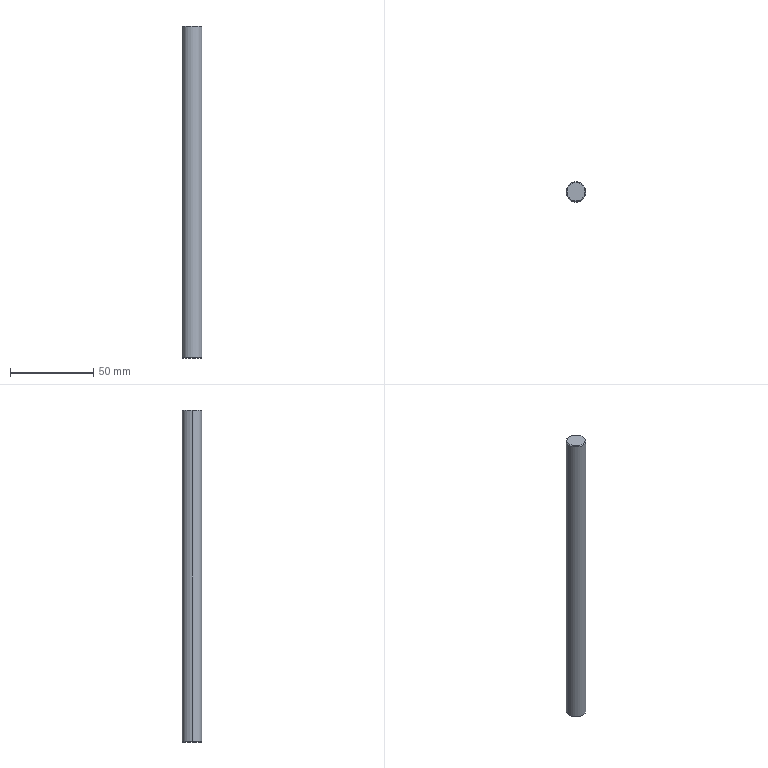Part | SolidWorks | features Chamfer 1, Extrusion 1 | 1 solid | 8 faces | box 12 x 12 x 200 mm | volume 22610 mm3 | cone 4 | cylinder 2 | plane 2 | commonest cylinder face diameters 12 x2
STEP:
#1=CARTESIAN_POINT('',(5.5,0.,100.));
#2=VERTEX_POINT('',#1);
#3=CARTESIAN_POINT('',(-5.5,0.,100.));
#4=VERTEX_POINT('',#3);
#5=CARTESIAN_POINT('',(0.,0.,100.));
#6=DIRECTION('',(0.,0.,1.));
#7=DIRECTION('',(1.,0.,0.));
#8=AXIS2_PLACEMENT_3D('',#5,#6,#7);
#9=CIRCLE('',#8,5.5);
#10=EDGE_CURVE('',#2,#4,#9,.T.);
#11=ORIENTED_EDGE('',*,*,#10,.F.);
#12=CARTESIAN_POINT('',(6.,0.,99.5));
#13=VERTEX_POINT('',#12);
#14=CARTESIAN_POINT('',(5.5,0.,100.));
#15=DIRECTION('',(0.7071,0.,-0.7071));
#16=VECTOR('',#15,1000.);
#17=LINE('',#14,#16);
#18=EDGE_CURVE('',#2,#13,#17,.T.);
#19=ORIENTED_EDGE('',*,*,#18,.T.);
#20=CARTESIAN_POINT('',(-6.,0.,99.5));
#21=VERTEX_POINT('',#20);
#22=CARTESIAN_POINT('',(0.,0.,99.5));
#23=DIRECTION('',(0.,0.,-1.));
#24=DIRECTION('',(1.,0.,0.));
#25=AXIS2_PLACEMENT_3D('',#22,#23,#24);
#26=CIRCLE('',#25,6.);
#27=EDGE_CURVE('',#21,#13,#26,.T.);
#28=ORIENTED_EDGE('',*,*,#27,.F.);
#29=CARTESIAN_POINT('',(-5.5,0.,100.));
#30=DIRECTION('',(-0.7071,0.,-0.7071));
#31=VECTOR('',#30,1000.);
#32=LINE('',#29,#31);
#33=EDGE_CURVE('',#4,#21,#32,.T.);
#34=ORIENTED_EDGE('',*,*,#33,.F.);
#35=EDGE_LOOP('',(#11,#19,#28,#34));
#36=FACE_OUTER_BOUND('',#35,.T.);
#37=CARTESIAN_POINT('',(0.,0.,100.));
#38=DIRECTION('',(0.,0.,-1.));
#39=DIRECTION('',(-1.,0.,0.));
#40=AXIS2_PLACEMENT_3D('',#37,#38,#39);
#41=CONICAL_SURFACE('',#40,5.5,0.7854);
#42=ADVANCED_FACE('',(#36),#41,.T.);
#43=CARTESIAN_POINT('',(-5.5,0.,-100.));
#44=VERTEX_POINT('',#43);
#45=CARTESIAN_POINT('',(5.5,0.,-100.));
#46=VERTEX_POINT('',#45);
#47=CARTESIAN_POINT('',(0.,0.,-100.));
#48=DIRECTION('',(0.,0.,-1.));
#49=DIRECTION('',(1.,0.,0.));
#50=AXIS2_PLACEMENT_3D('',#47,#48,#49);
#51=CIRCLE('',#50,5.5);
#52=EDGE_CURVE('',#44,#46,#51,.T.);
#53=ORIENTED_EDGE('',*,*,#52,.F.);
#54=CARTESIAN_POINT('',(-6.,0.,-99.5));
#55=VERTEX_POINT('',#54);
#56=CARTESIAN_POINT('',(-6.,0.,-99.5));
#57=DIRECTION('',(-0.7071,0.,0.7071));
#58=VECTOR('',#57,1000.);
#59=LINE('',#56,#58);
#60=EDGE_CURVE('',#44,#55,#59,.T.);
#61=ORIENTED_EDGE('',*,*,#60,.T.);
#62=CARTESIAN_POINT('',(6.,0.,-99.5));
#63=VERTEX_POINT('',#62);
#64=CARTESIAN_POINT('',(0.,0.,-99.5));
#65=DIRECTION('',(0.,0.,1.));
#66=DIRECTION('',(1.,0.,0.));
#67=AXIS2_PLACEMENT_3D('',#64,#65,#66);
#68=CIRCLE('',#67,6.);
#69=EDGE_CURVE('',#63,#55,#68,.T.);
#70=ORIENTED_EDGE('',*,*,#69,.F.);
#71=CARTESIAN_POINT('',(6.,0.,-99.5));
#72=DIRECTION('',(0.7071,0.,0.7071));
#73=VECTOR('',#72,1000.);
#74=LINE('',#71,#73);
#75=EDGE_CURVE('',#46,#63,#74,.T.);
#76=ORIENTED_EDGE('',*,*,#75,.F.);
#77=EDGE_LOOP('',(#53,#61,#70,#76));
#78=FACE_OUTER_BOUND('',#77,.T.);
#79=CARTESIAN_POINT('',(0.,0.,-99.5));
#80=DIRECTION('',(0.,0.,1.));
#81=DIRECTION('',(1.,0.,0.));
#82=AXIS2_PLACEMENT_3D('',#79,#80,#81);
#83=CONICAL_SURFACE('',#82,6.,0.7854);
#84=ADVANCED_FACE('',(#78),#83,.T.);
#85=ORIENTED_EDGE('',*,*,#27,.T.);
#86=CARTESIAN_POINT('',(6.,0.,100.));
#87=DIRECTION('',(0.,0.,-1.));
#88=VECTOR('',#87,1000.);
#89=LINE('',#86,#88);
#90=EDGE_CURVE('',#13,#63,#89,.T.);
#91=ORIENTED_EDGE('',*,*,#90,.T.);
#92=ORIENTED_EDGE('',*,*,#69,.T.);
#93=CARTESIAN_POINT('',(-6.,0.,100.));
#94=DIRECTION('',(0.,0.,-1.));
#95=VECTOR('',#94,1000.);
#96=LINE('',#93,#95);
#97=EDGE_CURVE('',#21,#55,#96,.T.);
#98=ORIENTED_EDGE('',*,*,#97,.F.);
#99=EDGE_LOOP('',(#85,#91,#92,#98));
#100=FACE_OUTER_BOUND('',#99,.T.);
#101=CARTESIAN_POINT('',(0.,0.,100.));
#102=DIRECTION('',(0.,0.,-1.));
#103=DIRECTION('',(-1.,0.,0.));
#104=AXIS2_PLACEMENT_3D('',#101,#102,#103);
#105=CYLINDRICAL_SURFACE('',#104,6.);
#106=ADVANCED_FACE('',(#100),#105,.T.);
#107=ORIENTED_EDGE('',*,*,#90,.F.);
#108=CARTESIAN_POINT('',(0.,0.,99.5));
#109=DIRECTION('',(0.,0.,-1.));
#110=DIRECTION('',(1.,0.,0.));
#111=AXIS2_PLACEMENT_3D('',#108,#109,#110);
#112=CIRCLE('',#111,6.);
#113=EDGE_CURVE('',#13,#21,#112,.T.);
#114=ORIENTED_EDGE('',*,*,#113,.T.);
#115=ORIENTED_EDGE('',*,*,#97,.T.);
#116=CARTESIAN_POINT('',(0.,0.,-99.5));
#117=DIRECTION('',(0.,0.,1.));
#118=DIRECTION('',(1.,0.,0.));
#119=AXIS2_PLACEMENT_3D('',#116,#117,#118);
#120=CIRCLE('',#119,6.);
#121=EDGE_CURVE('',#55,#63,#120,.T.);
#122=ORIENTED_EDGE('',*,*,#121,.T.);
#123=EDGE_LOOP('',(#107,#114,#115,#122));
#124=FACE_OUTER_BOUND('',#123,.T.);
#125=CARTESIAN_POINT('',(0.,0.,100.));
#126=DIRECTION('',(0.,0.,-1.));
#127=DIRECTION('',(-1.,0.,0.));
#128=AXIS2_PLACEMENT_3D('',#125,#126,#127);
#129=CYLINDRICAL_SURFACE('',#128,6.);
#130=ADVANCED_FACE('',(#124),#129,.T.);
#131=CARTESIAN_POINT('',(0.,0.,100.));
#132=DIRECTION('',(0.,0.,1.));
#133=DIRECTION('',(1.,0.,0.));
#134=AXIS2_PLACEMENT_3D('',#131,#132,#133);
#135=CIRCLE('',#134,5.5);
#136=EDGE_CURVE('',#4,#2,#135,.T.);
#137=ORIENTED_EDGE('',*,*,#136,.T.);
#138=ORIENTED_EDGE('',*,*,#10,.T.);
#139=EDGE_LOOP('',(#137,#138));
#140=FACE_OUTER_BOUND('',#139,.T.);
#141=CARTESIAN_POINT('',(0.,0.,100.));
#142=DIRECTION('',(0.,0.,1.));
#143=DIRECTION('',(1.,0.,0.));
#144=AXIS2_PLACEMENT_3D('',#141,#142,#143);
#145=PLANE('',#144);
#146=ADVANCED_FACE('',(#140),#145,.T.);
#147=CARTESIAN_POINT('',(0.,0.,-100.));
#148=DIRECTION('',(0.,0.,-1.));
#149=DIRECTION('',(1.,0.,0.));
#150=AXIS2_PLACEMENT_3D('',#147,#148,#149);
#151=CIRCLE('',#150,5.5);
#152=EDGE_CURVE('',#46,#44,#151,.T.);
#153=ORIENTED_EDGE('',*,*,#152,.T.);
#154=ORIENTED_EDGE('',*,*,#52,.T.);
#155=EDGE_LOOP('',(#153,#154));
#156=FACE_OUTER_BOUND('',#155,.T.);
#157=CARTESIAN_POINT('',(0.,0.,-100.));
#158=DIRECTION('',(0.,0.,1.));
#159=DIRECTION('',(1.,0.,0.));
#160=AXIS2_PLACEMENT_3D('',#157,#158,#159);
#161=PLANE('',#160);
#162=ADVANCED_FACE('',(#156),#161,.F.);
#163=ORIENTED_EDGE('',*,*,#60,.F.);
#164=ORIENTED_EDGE('',*,*,#152,.F.);
#165=ORIENTED_EDGE('',*,*,#75,.T.);
#166=ORIENTED_EDGE('',*,*,#121,.F.);
#167=EDGE_LOOP('',(#163,#164,#165,#166));
#168=FACE_OUTER_BOUND('',#167,.T.);
#169=CARTESIAN_POINT('',(0.,0.,-99.5));
#170=DIRECTION('',(0.,0.,1.));
#171=DIRECTION('',(1.,0.,0.));
#172=AXIS2_PLACEMENT_3D('',#169,#170,#171);
#173=CONICAL_SURFACE('',#172,6.,0.7854);
#174=ADVANCED_FACE('',(#168),#173,.T.);
#175=ORIENTED_EDGE('',*,*,#18,.F.);
#176=ORIENTED_EDGE('',*,*,#136,.F.);
#177=ORIENTED_EDGE('',*,*,#33,.T.);
#178=ORIENTED_EDGE('',*,*,#113,.F.);
#179=EDGE_LOOP('',(#175,#176,#177,#178));
#180=FACE_OUTER_BOUND('',#179,.T.);
#181=CARTESIAN_POINT('',(0.,0.,100.));
#182=DIRECTION('',(0.,0.,-1.));
#183=DIRECTION('',(-1.,0.,0.));
#184=AXIS2_PLACEMENT_3D('',#181,#182,#183);
#185=CONICAL_SURFACE('',#184,5.5,0.7854);
#186=ADVANCED_FACE('',(#180),#185,.T.);
#187=CLOSED_SHELL('',(#42,#84,#106,#130,#146,#162,#174,#186));
#188=MANIFOLD_SOLID_BREP('',#187);
#189=CARTESIAN_POINT('',(0.,0.,0.));
#190=DIRECTION('',(0.,0.,1.));
#191=DIRECTION('',(1.,0.,0.));
#192=AXIS2_PLACEMENT_3D('',#189,#190,#191);
#193=(LENGTH_UNIT()NAMED_UNIT(*)SI_UNIT(.MILLI.,.METRE.));
#194=UNCERTAINTY_MEASURE_WITH_UNIT(LENGTH_MEASURE(0.00001),#193,'','');
#195=(NAMED_UNIT(*)PLANE_ANGLE_UNIT()SI_UNIT($,.RADIAN.));
#196=(NAMED_UNIT(*)SI_UNIT($,.STERADIAN.)SOLID_ANGLE_UNIT());
#197=(GEOMETRIC_REPRESENTATION_CONTEXT(3)GLOBAL_UNCERTAINTY_ASSIGNED_CONTEXT((#194))GLOBAL_UNIT_ASSIGNED_CONTEXT((#193,#195,#196))REPRESENTATION_CONTEXT('',''));
#198=ADVANCED_BREP_SHAPE_REPRESENTATION('',(#188,#192),#197);